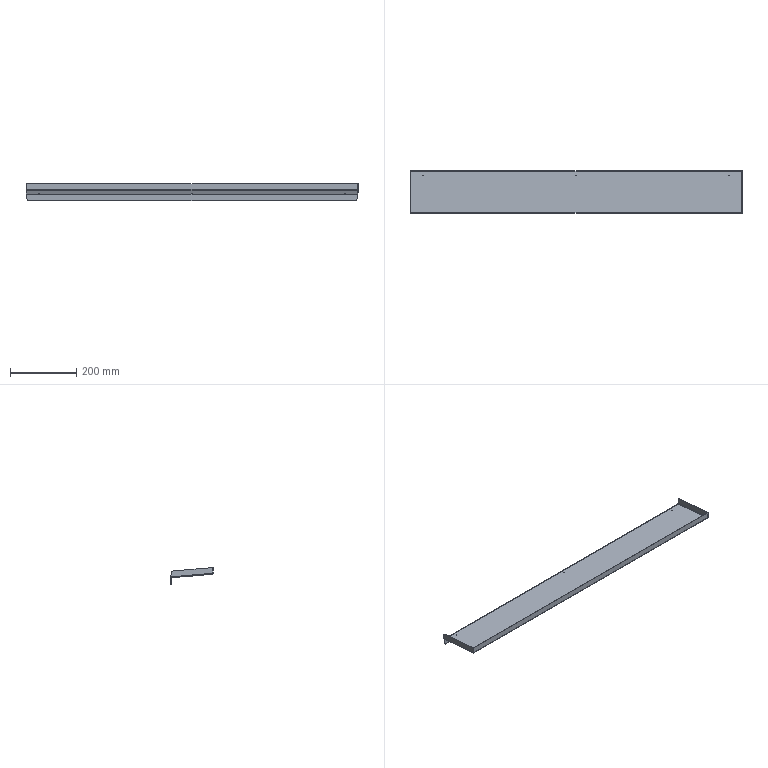Part | NX | features solid 2 | 1 solid | 56 faces | box 1000 x 127.951 x 51.256 mm | volume 254380 mm3 | plane 36 | cylinder 18 | spline 2 | commonest cylinder face diameters 2 x6 3 x4 6 x4 10 x4